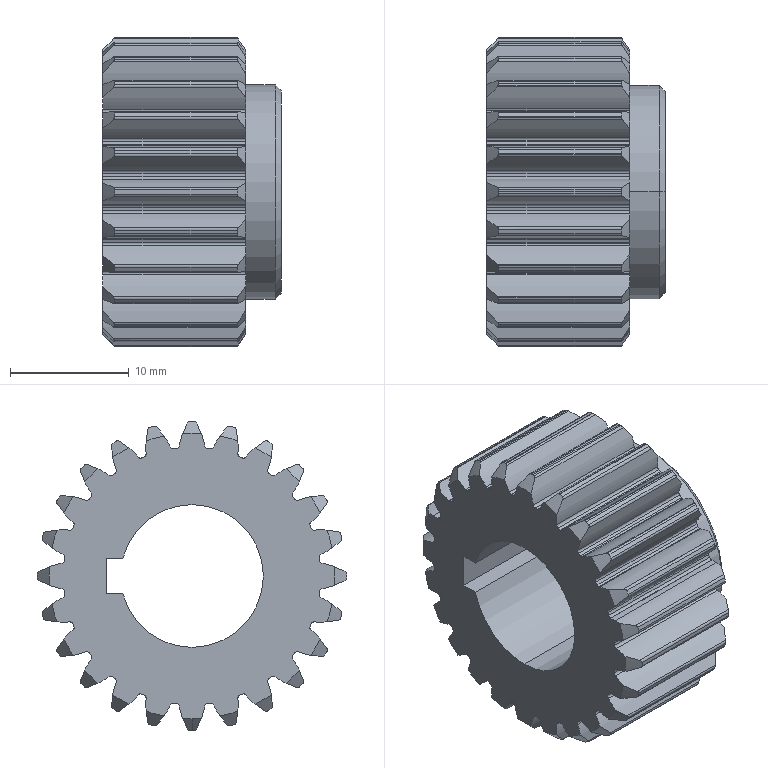Part | SolidWorks | features BaseBody 1 | 1 solid | 276 faces | box 15 x 26 x 26 mm | volume 4375 mm3 | cylinder 218 | cone 52 | plane 6 | commonest cylinder face diameters 0.5 x114 13.128 x50 26 x25 21.6 x24 12 x3 18 x2